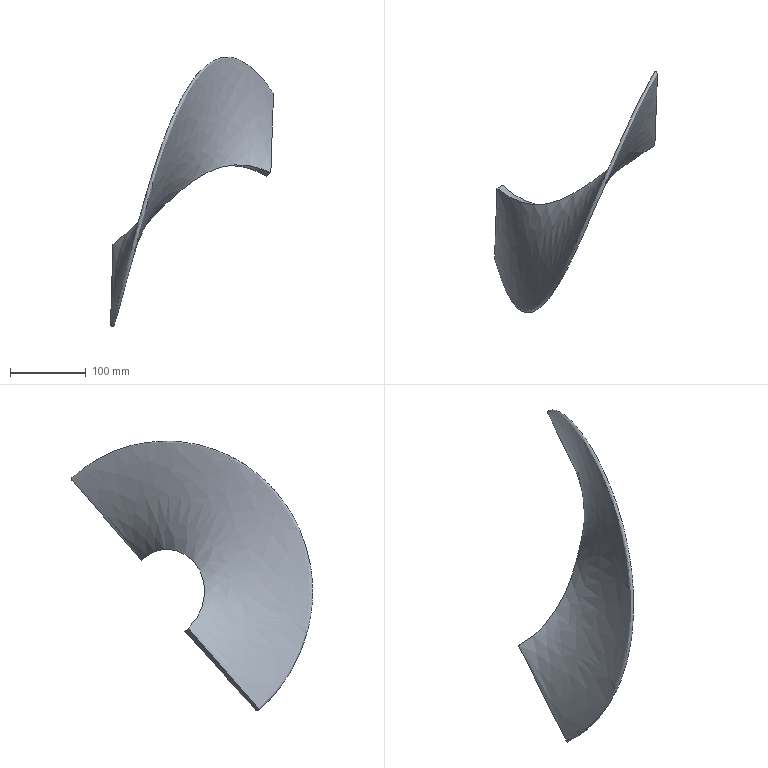Part | STEP file | Input 35 | 1 solid | 4 faces | box 215.218 x 318.536 x 356.446 mm | volume 751213 mm3 | spline 2 | plane 2